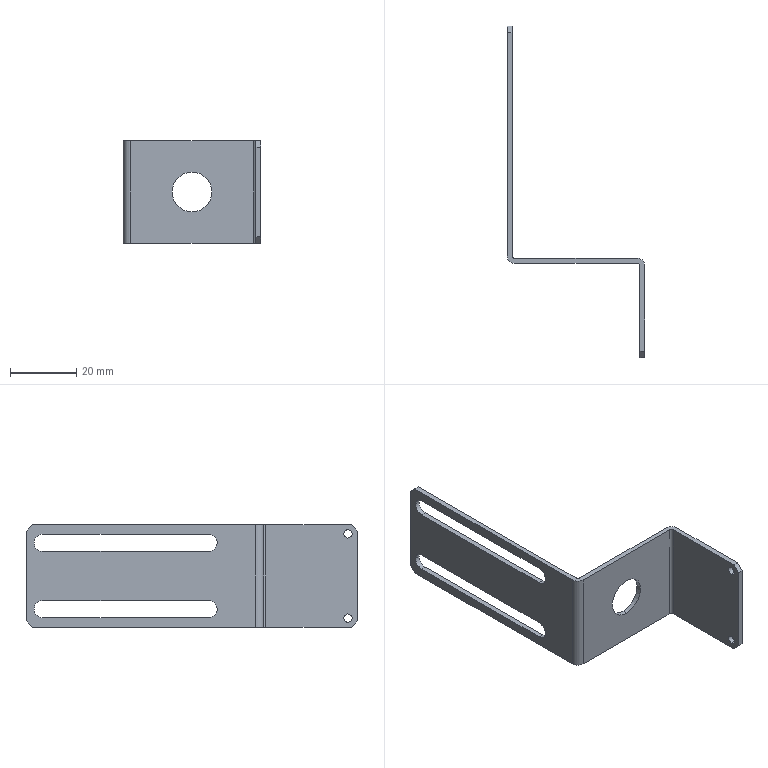Part | SolidWorks | features BaseBody 1 | 1 solid | 34 faces | box 41.5 x 100 x 31 mm | volume 5411 mm3 | plane 18 | cylinder 16 | commonest cylinder face diameters 5.2 x6 2.5 x4 1.473 x2 4.473 x2 12 x2
STEP:
#1=CARTESIAN_POINT('',(40.,-27.,4.05));
#2=VERTEX_POINT('',#1);
#3=CARTESIAN_POINT('',(40.,-27.,1.55));
#4=VERTEX_POINT('',#3);
#5=CARTESIAN_POINT('',(40.,-27.,2.8));
#6=DIRECTION('',(1.,0.,0.));
#7=DIRECTION('',(0.,1.,0.));
#8=AXIS2_PLACEMENT_3D('',#5,#6,#7);
#9=CIRCLE('',#8,1.25);
#10=EDGE_CURVE('',#2,#4,#9,.T.);
#11=ORIENTED_EDGE('',*,*,#10,.T.);
#12=CARTESIAN_POINT('',(38.5,-27.,1.55));
#13=VERTEX_POINT('',#12);
#14=CARTESIAN_POINT('',(38.5,-27.,1.55));
#15=DIRECTION('',(-1.,0.,0.));
#16=VECTOR('',#15,1000.);
#17=LINE('',#14,#16);
#18=EDGE_CURVE('',#4,#13,#17,.T.);
#19=ORIENTED_EDGE('',*,*,#18,.T.);
#20=CARTESIAN_POINT('',(38.5,-27.,4.05));
#21=VERTEX_POINT('',#20);
#22=CARTESIAN_POINT('',(38.5,-27.,2.8));
#23=DIRECTION('',(-1.,0.,0.));
#24=DIRECTION('',(0.,0.,1.));
#25=AXIS2_PLACEMENT_3D('',#22,#23,#24);
#26=CIRCLE('',#25,1.25);
#27=EDGE_CURVE('',#13,#21,#26,.T.);
#28=ORIENTED_EDGE('',*,*,#27,.T.);
#29=CARTESIAN_POINT('',(38.5,-27.,4.05));
#30=DIRECTION('',(-1.,0.,0.));
#31=VECTOR('',#30,1000.);
#32=LINE('',#29,#31);
#33=EDGE_CURVE('',#2,#21,#32,.T.);
#34=ORIENTED_EDGE('',*,*,#33,.F.);
#35=EDGE_LOOP('',(#11,#19,#28,#34));
#36=FACE_OUTER_BOUND('',#35,.T.);
#37=CARTESIAN_POINT('',(38.5,-27.,2.8));
#38=DIRECTION('',(-1.,0.,0.));
#39=DIRECTION('',(0.,0.,1.));
#40=AXIS2_PLACEMENT_3D('',#37,#38,#39);
#41=CYLINDRICAL_SURFACE('',#40,1.25);
#42=ADVANCED_FACE('',(#36),#41,.F.);
#43=CARTESIAN_POINT('',(40.,-27.,29.45));
#44=VERTEX_POINT('',#43);
#45=CARTESIAN_POINT('',(40.,-27.,26.95));
#46=VERTEX_POINT('',#45);
#47=CARTESIAN_POINT('',(40.,-27.,28.2));
#48=DIRECTION('',(1.,0.,0.));
#49=DIRECTION('',(0.,1.,0.));
#50=AXIS2_PLACEMENT_3D('',#47,#48,#49);
#51=CIRCLE('',#50,1.25);
#52=EDGE_CURVE('',#44,#46,#51,.T.);
#53=ORIENTED_EDGE('',*,*,#52,.T.);
#54=CARTESIAN_POINT('',(38.5,-27.,26.95));
#55=VERTEX_POINT('',#54);
#56=CARTESIAN_POINT('',(38.5,-27.,26.95));
#57=DIRECTION('',(-1.,0.,0.));
#58=VECTOR('',#57,1000.);
#59=LINE('',#56,#58);
#60=EDGE_CURVE('',#46,#55,#59,.T.);
#61=ORIENTED_EDGE('',*,*,#60,.T.);
#62=CARTESIAN_POINT('',(38.5,-27.,29.45));
#63=VERTEX_POINT('',#62);
#64=CARTESIAN_POINT('',(38.5,-27.,28.2));
#65=DIRECTION('',(-1.,0.,0.));
#66=DIRECTION('',(0.,0.,1.));
#67=AXIS2_PLACEMENT_3D('',#64,#65,#66);
#68=CIRCLE('',#67,1.25);
#69=EDGE_CURVE('',#55,#63,#68,.T.);
#70=ORIENTED_EDGE('',*,*,#69,.T.);
#71=CARTESIAN_POINT('',(38.5,-27.,29.45));
#72=DIRECTION('',(-1.,0.,0.));
#73=VECTOR('',#72,1000.);
#74=LINE('',#71,#73);
#75=EDGE_CURVE('',#44,#63,#74,.T.);
#76=ORIENTED_EDGE('',*,*,#75,.F.);
#77=EDGE_LOOP('',(#53,#61,#70,#76));
#78=FACE_OUTER_BOUND('',#77,.T.);
#79=CARTESIAN_POINT('',(38.5,-27.,28.2));
#80=DIRECTION('',(-1.,0.,0.));
#81=DIRECTION('',(0.,0.,1.));
#82=AXIS2_PLACEMENT_3D('',#79,#80,#81);
#83=CYLINDRICAL_SURFACE('',#82,1.25);
#84=ADVANCED_FACE('',(#78),#83,.F.);
#85=CARTESIAN_POINT('',(19.25,-1.5,9.5));
#86=VERTEX_POINT('',#85);
#87=CARTESIAN_POINT('',(19.25,-1.5,21.5));
#88=VERTEX_POINT('',#87);
#89=CARTESIAN_POINT('',(19.25,-1.5,15.5));
#90=DIRECTION('',(0.,1.,0.));
#91=DIRECTION('',(0.,0.,1.));
#92=AXIS2_PLACEMENT_3D('',#89,#90,#91);
#93=CIRCLE('',#92,6.);
#94=EDGE_CURVE('',#86,#88,#93,.T.);
#95=ORIENTED_EDGE('',*,*,#94,.F.);
#96=CARTESIAN_POINT('',(19.25,0.,9.5));
#97=VERTEX_POINT('',#96);
#98=CARTESIAN_POINT('',(19.25,-10.,9.5));
#99=DIRECTION('',(0.,1.,0.));
#100=VECTOR('',#99,1000.);
#101=LINE('',#98,#100);
#102=EDGE_CURVE('',#86,#97,#101,.T.);
#103=ORIENTED_EDGE('',*,*,#102,.T.);
#104=CARTESIAN_POINT('',(19.25,0.,21.5));
#105=VERTEX_POINT('',#104);
#106=CARTESIAN_POINT('',(19.25,0.,15.5));
#107=DIRECTION('',(0.,1.,0.));
#108=DIRECTION('',(0.,0.,1.));
#109=AXIS2_PLACEMENT_3D('',#106,#107,#108);
#110=CIRCLE('',#109,6.);
#111=EDGE_CURVE('',#97,#105,#110,.T.);
#112=ORIENTED_EDGE('',*,*,#111,.T.);
#113=CARTESIAN_POINT('',(19.25,-10.,21.5));
#114=DIRECTION('',(0.,1.,0.));
#115=VECTOR('',#114,1000.);
#116=LINE('',#113,#115);
#117=EDGE_CURVE('',#88,#105,#116,.T.);
#118=ORIENTED_EDGE('',*,*,#117,.F.);
#119=EDGE_LOOP('',(#95,#103,#112,#118));
#120=FACE_OUTER_BOUND('',#119,.T.);
#121=CARTESIAN_POINT('',(19.25,-10.,15.5));
#122=DIRECTION('',(0.,1.,0.));
#123=DIRECTION('',(0.,0.,1.));
#124=AXIS2_PLACEMENT_3D('',#121,#122,#123);
#125=CYLINDRICAL_SURFACE('',#124,6.);
#126=ADVANCED_FACE('',(#120),#125,.F.);
#127=CARTESIAN_POINT('',(-1.5,67.6,5.5));
#128=VERTEX_POINT('',#127);
#129=CARTESIAN_POINT('',(-1.5,65.,8.1));
#130=VERTEX_POINT('',#129);
#131=CARTESIAN_POINT('',(-1.5,65.,5.5));
#132=DIRECTION('',(1.,0.,0.));
#133=DIRECTION('',(0.,1.,0.));
#134=AXIS2_PLACEMENT_3D('',#131,#132,#133);
#135=CIRCLE('',#134,2.6);
#136=EDGE_CURVE('',#128,#130,#135,.T.);
#137=ORIENTED_EDGE('',*,*,#136,.F.);
#138=CARTESIAN_POINT('',(0.,67.6,5.5));
#139=VERTEX_POINT('',#138);
#140=CARTESIAN_POINT('',(-10.,67.6,5.5));
#141=DIRECTION('',(1.,0.,0.));
#142=VECTOR('',#141,1000.);
#143=LINE('',#140,#142);
#144=EDGE_CURVE('',#128,#139,#143,.T.);
#145=ORIENTED_EDGE('',*,*,#144,.T.);
#146=CARTESIAN_POINT('',(0.,65.,8.1));
#147=VERTEX_POINT('',#146);
#148=CARTESIAN_POINT('',(0.,65.,5.5));
#149=DIRECTION('',(1.,0.,0.));
#150=DIRECTION('',(0.,1.,0.));
#151=AXIS2_PLACEMENT_3D('',#148,#149,#150);
#152=CIRCLE('',#151,2.6);
#153=EDGE_CURVE('',#139,#147,#152,.T.);
#154=ORIENTED_EDGE('',*,*,#153,.T.);
#155=CARTESIAN_POINT('',(-10.,65.,8.1));
#156=DIRECTION('',(1.,0.,0.));
#157=VECTOR('',#156,1000.);
#158=LINE('',#155,#157);
#159=EDGE_CURVE('',#130,#147,#158,.T.);
#160=ORIENTED_EDGE('',*,*,#159,.F.);
#161=EDGE_LOOP('',(#137,#145,#154,#160));
#162=FACE_OUTER_BOUND('',#161,.T.);
#163=CARTESIAN_POINT('',(-10.,65.,5.5));
#164=DIRECTION('',(1.,0.,0.));
#165=DIRECTION('',(0.,1.,0.));
#166=AXIS2_PLACEMENT_3D('',#163,#164,#165);
#167=CYLINDRICAL_SURFACE('',#166,2.6);
#168=ADVANCED_FACE('',(#162),#167,.F.);
#169=CARTESIAN_POINT('',(-1.5,67.6,25.5));
#170=VERTEX_POINT('',#169);
#171=CARTESIAN_POINT('',(-1.5,65.,28.1));
#172=VERTEX_POINT('',#171);
#173=CARTESIAN_POINT('',(-1.5,65.,25.5));
#174=DIRECTION('',(1.,0.,0.));
#175=DIRECTION('',(0.,1.,0.));
#176=AXIS2_PLACEMENT_3D('',#173,#174,#175);
#177=CIRCLE('',#176,2.6);
#178=EDGE_CURVE('',#170,#172,#177,.T.);
#179=ORIENTED_EDGE('',*,*,#178,.F.);
#180=CARTESIAN_POINT('',(0.,67.6,25.5));
#181=VERTEX_POINT('',#180);
#182=CARTESIAN_POINT('',(-10.,67.6,25.5));
#183=DIRECTION('',(1.,0.,0.));
#184=VECTOR('',#183,1000.);
#185=LINE('',#182,#184);
#186=EDGE_CURVE('',#170,#181,#185,.T.);
#187=ORIENTED_EDGE('',*,*,#186,.T.);
#188=CARTESIAN_POINT('',(0.,65.,28.1));
#189=VERTEX_POINT('',#188);
#190=CARTESIAN_POINT('',(0.,65.,25.5));
#191=DIRECTION('',(1.,0.,0.));
#192=DIRECTION('',(0.,1.,0.));
#193=AXIS2_PLACEMENT_3D('',#190,#191,#192);
#194=CIRCLE('',#193,2.6);
#195=EDGE_CURVE('',#181,#189,#194,.T.);
#196=ORIENTED_EDGE('',*,*,#195,.T.);
#197=CARTESIAN_POINT('',(-10.,65.,28.1));
#198=DIRECTION('',(1.,0.,0.));
#199=VECTOR('',#198,1000.);
#200=LINE('',#197,#199);
#201=EDGE_CURVE('',#172,#189,#200,.T.);
#202=ORIENTED_EDGE('',*,*,#201,.F.);
#203=EDGE_LOOP('',(#179,#187,#196,#202));
#204=FACE_OUTER_BOUND('',#203,.T.);
#205=CARTESIAN_POINT('',(-10.,65.,25.5));
#206=DIRECTION('',(1.,0.,0.));
#207=DIRECTION('',(0.,1.,0.));
#208=AXIS2_PLACEMENT_3D('',#205,#206,#207);
#209=CYLINDRICAL_SURFACE('',#208,2.6);
#210=ADVANCED_FACE('',(#204),#209,.F.);
#211=CARTESIAN_POINT('',(40.,-28.,31.));
#212=VERTEX_POINT('',#211);
#213=CARTESIAN_POINT('',(40.,-30.,29.));
#214=VERTEX_POINT('',#213);
#215=CARTESIAN_POINT('',(40.,-14.,45.));
#216=DIRECTION('',(0.,-0.7071,-0.7071));
#217=VECTOR('',#216,1000.);
#218=LINE('',#215,#217);
#219=EDGE_CURVE('',#212,#214,#218,.T.);
#220=ORIENTED_EDGE('',*,*,#219,.F.);
#221=CARTESIAN_POINT('',(38.5,-28.,31.));
#222=VERTEX_POINT('',#221);
#223=CARTESIAN_POINT('',(37.763,-28.,31.));
#224=DIRECTION('',(1.,0.,0.));
#225=VECTOR('',#224,1000.);
#226=LINE('',#223,#225);
#227=EDGE_CURVE('',#222,#212,#226,.T.);
#228=ORIENTED_EDGE('',*,*,#227,.F.);
#229=CARTESIAN_POINT('',(38.5,-30.,29.));
#230=VERTEX_POINT('',#229);
#231=CARTESIAN_POINT('',(38.5,-30.,29.));
#232=DIRECTION('',(0.,0.7071,0.7071));
#233=VECTOR('',#232,1000.);
#234=LINE('',#231,#233);
#235=EDGE_CURVE('',#230,#222,#234,.T.);
#236=ORIENTED_EDGE('',*,*,#235,.F.);
#237=CARTESIAN_POINT('',(40.,-30.,29.));
#238=DIRECTION('',(-1.,0.,0.));
#239=VECTOR('',#238,1000.);
#240=LINE('',#237,#239);
#241=EDGE_CURVE('',#214,#230,#240,.T.);
#242=ORIENTED_EDGE('',*,*,#241,.F.);
#243=EDGE_LOOP('',(#220,#228,#236,#242));
#244=FACE_OUTER_BOUND('',#243,.T.);
#245=CARTESIAN_POINT('',(40.,-30.,29.));
#246=DIRECTION('',(0.,0.7071,-0.7071));
#247=DIRECTION('',(-1.,0.,0.));
#248=AXIS2_PLACEMENT_3D('',#245,#246,#247);
#249=PLANE('',#248);
#250=ADVANCED_FACE('',(#244),#249,.F.);
#251=CARTESIAN_POINT('',(40.,-30.,2.));
#252=VERTEX_POINT('',#251);
#253=CARTESIAN_POINT('',(40.,-28.,0.));
#254=VERTEX_POINT('',#253);
#255=CARTESIAN_POINT('',(40.,-29.5,1.5));
#256=DIRECTION('',(0.,0.7071,-0.7071));
#257=VECTOR('',#256,1000.);
#258=LINE('',#255,#257);
#259=EDGE_CURVE('',#252,#254,#258,.T.);
#260=ORIENTED_EDGE('',*,*,#259,.F.);
#261=CARTESIAN_POINT('',(38.5,-30.,2.));
#262=VERTEX_POINT('',#261);
#263=CARTESIAN_POINT('',(40.,-30.,2.));
#264=DIRECTION('',(1.,0.,0.));
#265=VECTOR('',#264,1000.);
#266=LINE('',#263,#265);
#267=EDGE_CURVE('',#262,#252,#266,.T.);
#268=ORIENTED_EDGE('',*,*,#267,.F.);
#269=CARTESIAN_POINT('',(38.5,-28.,0.));
#270=VERTEX_POINT('',#269);
#271=CARTESIAN_POINT('',(38.5,-28.,0.));
#272=DIRECTION('',(0.,-0.7071,0.7071));
#273=VECTOR('',#272,1000.);
#274=LINE('',#271,#273);
#275=EDGE_CURVE('',#270,#262,#274,.T.);
#276=ORIENTED_EDGE('',*,*,#275,.F.);
#277=CARTESIAN_POINT('',(38.5,-28.,0.));
#278=DIRECTION('',(-1.,0.,0.));
#279=VECTOR('',#278,1000.);
#280=LINE('',#277,#279);
#281=EDGE_CURVE('',#254,#270,#280,.T.);
#282=ORIENTED_EDGE('',*,*,#281,.F.);
#283=EDGE_LOOP('',(#260,#268,#276,#282));
#284=FACE_OUTER_BOUND('',#283,.T.);
#285=CARTESIAN_POINT('',(37.763,-28.,0.));
#286=DIRECTION('',(0.,-0.7071,-0.7071));
#287=DIRECTION('',(0.,-0.7071,0.7071));
#288=AXIS2_PLACEMENT_3D('',#285,#286,#287);
#289=PLANE('',#288);
#290=ADVANCED_FACE('',(#284),#289,.T.);
#291=CARTESIAN_POINT('',(-1.5,68.,31.));
#292=VERTEX_POINT('',#291);
#293=CARTESIAN_POINT('',(-1.5,70.,29.));
#294=VERTEX_POINT('',#293);
#295=CARTESIAN_POINT('',(-1.5,70.,29.));
#296=DIRECTION('',(0.,0.7071,-0.7071));
#297=VECTOR('',#296,1000.);
#298=LINE('',#295,#297);
#299=EDGE_CURVE('',#292,#294,#298,.T.);
#300=ORIENTED_EDGE('',*,*,#299,.F.);
#301=CARTESIAN_POINT('',(0.,68.,31.));
#302=VERTEX_POINT('',#301);
#303=CARTESIAN_POINT('',(37.763,68.,31.));
#304=DIRECTION('',(-1.,0.,0.));
#305=VECTOR('',#304,1000.);
#306=LINE('',#303,#305);
#307=EDGE_CURVE('',#302,#292,#306,.T.);
#308=ORIENTED_EDGE('',*,*,#307,.F.);
#309=CARTESIAN_POINT('',(0.,70.,29.));
#310=VERTEX_POINT('',#309);
#311=CARTESIAN_POINT('',(0.,69.,30.));
#312=DIRECTION('',(0.,-0.7071,0.7071));
#313=VECTOR('',#312,1000.);
#314=LINE('',#311,#313);
#315=EDGE_CURVE('',#310,#302,#314,.T.);
#316=ORIENTED_EDGE('',*,*,#315,.F.);
#317=CARTESIAN_POINT('',(-1.5,70.,29.));
#318=DIRECTION('',(1.,0.,0.));
#319=VECTOR('',#318,1000.);
#320=LINE('',#317,#319);
#321=EDGE_CURVE('',#294,#310,#320,.T.);
#322=ORIENTED_EDGE('',*,*,#321,.F.);
#323=EDGE_LOOP('',(#300,#308,#316,#322));
#324=FACE_OUTER_BOUND('',#323,.T.);
#325=CARTESIAN_POINT('',(-1.5,70.,29.));
#326=DIRECTION('',(0.,-0.7071,-0.7071));
#327=DIRECTION('',(0.,-0.7071,0.7071));
#328=AXIS2_PLACEMENT_3D('',#325,#326,#327);
#329=PLANE('',#328);
#330=ADVANCED_FACE('',(#324),#329,.F.);
#331=CARTESIAN_POINT('',(-1.5,70.,2.));
#332=VERTEX_POINT('',#331);
#333=CARTESIAN_POINT('',(-1.5,68.,0.));
#334=VERTEX_POINT('',#333);
#335=CARTESIAN_POINT('',(-1.5,68.,0.));
#336=DIRECTION('',(0.,-0.7071,-0.7071));
#337=VECTOR('',#336,1000.);
#338=LINE('',#335,#337);
#339=EDGE_CURVE('',#332,#334,#338,.T.);
#340=ORIENTED_EDGE('',*,*,#339,.F.);
#341=CARTESIAN_POINT('',(0.,70.,2.));
#342=VERTEX_POINT('',#341);
#343=CARTESIAN_POINT('',(-1.5,70.,2.));
#344=DIRECTION('',(-1.,0.,0.));
#345=VECTOR('',#344,1000.);
#346=LINE('',#343,#345);
#347=EDGE_CURVE('',#342,#332,#346,.T.);
#348=ORIENTED_EDGE('',*,*,#347,.F.);
#349=CARTESIAN_POINT('',(0.,68.,0.));
#350=VERTEX_POINT('',#349);
#351=CARTESIAN_POINT('',(0.,84.5,16.5));
#352=DIRECTION('',(0.,0.7071,0.7071));
#353=VECTOR('',#352,1000.);
#354=LINE('',#351,#353);
#355=EDGE_CURVE('',#350,#342,#354,.T.);
#356=ORIENTED_EDGE('',*,*,#355,.F.);
#357=CARTESIAN_POINT('',(0.7366,68.,0.));
#358=DIRECTION('',(1.,0.,0.));
#359=VECTOR('',#358,1000.);
#360=LINE('',#357,#359);
#361=EDGE_CURVE('',#334,#350,#360,.T.);
#362=ORIENTED_EDGE('',*,*,#361,.F.);
#363=EDGE_LOOP('',(#340,#348,#356,#362));
#364=FACE_OUTER_BOUND('',#363,.T.);
#365=CARTESIAN_POINT('',(0.7366,68.,0.));
#366=DIRECTION('',(0.,-0.7071,0.7071));
#367=DIRECTION('',(-1.,0.,0.));
#368=AXIS2_PLACEMENT_3D('',#365,#366,#367);
#369=PLANE('',#368);
#370=ADVANCED_FACE('',(#364),#369,.F.);
#371=ORIENTED_EDGE('',*,*,#159,.T.);
#372=CARTESIAN_POINT('',(0.,15.,8.1));
#373=VERTEX_POINT('',#372);
#374=CARTESIAN_POINT('',(0.,65.,8.1));
#375=DIRECTION('',(0.,-1.,0.));
#376=VECTOR('',#375,1000.);
#377=LINE('',#374,#376);
#378=EDGE_CURVE('',#147,#373,#377,.T.);
#379=ORIENTED_EDGE('',*,*,#378,.T.);
#380=CARTESIAN_POINT('',(-1.5,15.,8.1));
#381=VERTEX_POINT('',#380);
#382=CARTESIAN_POINT('',(-10.,15.,8.1));
#383=DIRECTION('',(1.,0.,0.));
#384=VECTOR('',#383,1000.);
#385=LINE('',#382,#384);
#386=EDGE_CURVE('',#381,#373,#385,.T.);
#387=ORIENTED_EDGE('',*,*,#386,.F.);
#388=CARTESIAN_POINT('',(-1.5,70.,8.1));
#389=DIRECTION('',(0.,-1.,0.));
#390=VECTOR('',#389,1000.);
#391=LINE('',#388,#390);
#392=EDGE_CURVE('',#130,#381,#391,.T.);
#393=ORIENTED_EDGE('',*,*,#392,.F.);
#394=EDGE_LOOP('',(#371,#379,#387,#393));
#395=FACE_OUTER_BOUND('',#394,.T.);
#396=CARTESIAN_POINT('',(-10.,65.,8.1));
#397=DIRECTION('',(0.,0.,1.));
#398=DIRECTION('',(0.,-1.,0.));
#399=AXIS2_PLACEMENT_3D('',#396,#397,#398);
#400=PLANE('',#399);
#401=ADVANCED_FACE('',(#395),#400,.F.);
#402=ORIENTED_EDGE('',*,*,#386,.T.);
#403=CARTESIAN_POINT('',(0.,15.,2.9));
#404=VERTEX_POINT('',#403);
#405=CARTESIAN_POINT('',(0.,15.,5.5));
#406=DIRECTION('',(1.,0.,0.));
#407=DIRECTION('',(0.,1.,0.));
#408=AXIS2_PLACEMENT_3D('',#405,#406,#407);
#409=CIRCLE('',#408,2.6);
#410=EDGE_CURVE('',#373,#404,#409,.T.);
#411=ORIENTED_EDGE('',*,*,#410,.T.);
#412=CARTESIAN_POINT('',(-1.5,15.,2.9));
#413=VERTEX_POINT('',#412);
#414=CARTESIAN_POINT('',(-10.,15.,2.9));
#415=DIRECTION('',(1.,0.,0.));
#416=VECTOR('',#415,1000.);
#417=LINE('',#414,#416);
#418=EDGE_CURVE('',#413,#404,#417,.T.);
#419=ORIENTED_EDGE('',*,*,#418,.F.);
#420=CARTESIAN_POINT('',(-1.5,15.,5.5));
#421=DIRECTION('',(1.,0.,0.));
#422=DIRECTION('',(0.,1.,0.));
#423=AXIS2_PLACEMENT_3D('',#420,#421,#422);
#424=CIRCLE('',#423,2.6);
#425=EDGE_CURVE('',#381,#413,#424,.T.);
#426=ORIENTED_EDGE('',*,*,#425,.F.);
#427=EDGE_LOOP('',(#402,#411,#419,#426));
#428=FACE_OUTER_BOUND('',#427,.T.);
#429=CARTESIAN_POINT('',(-10.,15.,5.5));
#430=DIRECTION('',(1.,0.,0.));
#431=DIRECTION('',(0.,1.,0.));
#432=AXIS2_PLACEMENT_3D('',#429,#430,#431);
#433=CYLINDRICAL_SURFACE('',#432,2.6);
#434=ADVANCED_FACE('',(#428),#433,.F.);
#435=ORIENTED_EDGE('',*,*,#418,.T.);
#436=CARTESIAN_POINT('',(0.,65.,2.9));
#437=VERTEX_POINT('',#436);
#438=CARTESIAN_POINT('',(0.,65.,2.9));
#439=DIRECTION('',(0.,1.,0.));
#440=VECTOR('',#439,1000.);
#441=LINE('',#438,#440);
#442=EDGE_CURVE('',#404,#437,#441,.T.);
#443=ORIENTED_EDGE('',*,*,#442,.T.);
#444=CARTESIAN_POINT('',(-1.5,65.,2.9));
#445=VERTEX_POINT('',#444);
#446=CARTESIAN_POINT('',(-10.,65.,2.9));
#447=DIRECTION('',(1.,0.,0.));
#448=VECTOR('',#447,1000.);
#449=LINE('',#446,#448);
#450=EDGE_CURVE('',#445,#437,#449,.T.);
#451=ORIENTED_EDGE('',*,*,#450,.F.);
#452=CARTESIAN_POINT('',(-1.5,70.,2.9));
#453=DIRECTION('',(0.,1.,0.));
#454=VECTOR('',#453,1000.);
#455=LINE('',#452,#454);
#456=EDGE_CURVE('',#413,#445,#455,.T.);
#457=ORIENTED_EDGE('',*,*,#456,.F.);
#458=EDGE_LOOP('',(#435,#443,#451,#457));
#459=FACE_OUTER_BOUND('',#458,.T.);
#460=CARTESIAN_POINT('',(-10.,65.,2.9));
#461=DIRECTION('',(0.,0.,-1.));
#462=DIRECTION('',(-1.,0.,0.));
#463=AXIS2_PLACEMENT_3D('',#460,#461,#462);
#464=PLANE('',#463);
#465=ADVANCED_FACE('',(#459),#464,.F.);
#466=ORIENTED_EDGE('',*,*,#201,.T.);
#467=CARTESIAN_POINT('',(0.,15.,28.1));
#468=VERTEX_POINT('',#467);
#469=CARTESIAN_POINT('',(0.,65.,28.1));
#470=DIRECTION('',(0.,-1.,0.));
#471=VECTOR('',#470,1000.);
#472=LINE('',#469,#471);
#473=EDGE_CURVE('',#189,#468,#472,.T.);
#474=ORIENTED_EDGE('',*,*,#473,.T.);
#475=CARTESIAN_POINT('',(-1.5,15.,28.1));
#476=VERTEX_POINT('',#475);
#477=CARTESIAN_POINT('',(-10.,15.,28.1));
#478=DIRECTION('',(1.,0.,0.));
#479=VECTOR('',#478,1000.);
#480=LINE('',#477,#479);
#481=EDGE_CURVE('',#476,#468,#480,.T.);
#482=ORIENTED_EDGE('',*,*,#481,.F.);
#483=CARTESIAN_POINT('',(-1.5,70.,28.1));
#484=DIRECTION('',(0.,-1.,0.));
#485=VECTOR('',#484,1000.);
#486=LINE('',#483,#485);
#487=EDGE_CURVE('',#172,#476,#486,.T.);
#488=ORIENTED_EDGE('',*,*,#487,.F.);
#489=EDGE_LOOP('',(#466,#474,#482,#488));
#490=FACE_OUTER_BOUND('',#489,.T.);
#491=CARTESIAN_POINT('',(-10.,65.,28.1));
#492=DIRECTION('',(0.,0.,1.));
#493=DIRECTION('',(0.,-1.,0.));
#494=AXIS2_PLACEMENT_3D('',#491,#492,#493);
#495=PLANE('',#494);
#496=ADVANCED_FACE('',(#490),#495,.F.);
#497=ORIENTED_EDGE('',*,*,#481,.T.);
#498=CARTESIAN_POINT('',(0.,15.,22.9));
#499=VERTEX_POINT('',#498);
#500=CARTESIAN_POINT('',(0.,15.,25.5));
#501=DIRECTION('',(1.,0.,0.));
#502=DIRECTION('',(0.,1.,0.));
#503=AXIS2_PLACEMENT_3D('',#500,#501,#502);
#504=CIRCLE('',#503,2.6);
#505=EDGE_CURVE('',#468,#499,#504,.T.);
#506=ORIENTED_EDGE('',*,*,#505,.T.);
#507=CARTESIAN_POINT('',(-1.5,15.,22.9));
#508=VERTEX_POINT('',#507);
#509=CARTESIAN_POINT('',(-10.,15.,22.9));
#510=DIRECTION('',(1.,0.,0.));
#511=VECTOR('',#510,1000.);
#512=LINE('',#509,#511);
#513=EDGE_CURVE('',#508,#499,#512,.T.);
#514=ORIENTED_EDGE('',*,*,#513,.F.);
#515=CARTESIAN_POINT('',(-1.5,15.,25.5));
#516=DIRECTION('',(1.,0.,0.));
#517=DIRECTION('',(0.,1.,0.));
#518=AXIS2_PLACEMENT_3D('',#515,#516,#517);
#519=CIRCLE('',#518,2.6);
#520=EDGE_CURVE('',#476,#508,#519,.T.);
#521=ORIENTED_EDGE('',*,*,#520,.F.);
#522=EDGE_LOOP('',(#497,#506,#514,#521));
#523=FACE_OUTER_BOUND('',#522,.T.);
#524=CARTESIAN_POINT('',(-10.,15.,25.5));
#525=DIRECTION('',(1.,0.,0.));
#526=DIRECTION('',(0.,1.,0.));
#527=AXIS2_PLACEMENT_3D('',#524,#525,#526);
#528=CYLINDRICAL_SURFACE('',#527,2.6);
#529=ADVANCED_FACE('',(#523),#528,.F.);
#530=ORIENTED_EDGE('',*,*,#513,.T.);
#531=CARTESIAN_POINT('',(0.,65.,22.9));
#532=VERTEX_POINT('',#531);
#533=CARTESIAN_POINT('',(0.,65.,22.9));
#534=DIRECTION('',(0.,1.,0.));
#535=VECTOR('',#534,1000.);
#536=LINE('',#533,#535);
#537=EDGE_CURVE('',#499,#532,#536,.T.);
#538=ORIENTED_EDGE('',*,*,#537,.T.);
#539=CARTESIAN_POINT('',(-1.5,65.,22.9));
#540=VERTEX_POINT('',#539);
#541=CARTESIAN_POINT('',(-10.,65.,22.9));
#542=DIRECTION('',(1.,0.,0.));
#543=VECTOR('',#542,1000.);
#544=LINE('',#541,#543);
#545=EDGE_CURVE('',#540,#532,#544,.T.);
#546=ORIENTED_EDGE('',*,*,#545,.F.);
#547=CARTESIAN_POINT('',(-1.5,70.,22.9));
#548=DIRECTION('',(0.,1.,0.));
#549=VECTOR('',#548,1000.);
#550=LINE('',#547,#549);
#551=EDGE_CURVE('',#508,#540,#550,.T.);
#552=ORIENTED_EDGE('',*,*,#551,.F.);
#553=EDGE_LOOP('',(#530,#538,#546,#552));
#554=FACE_OUTER_BOUND('',#553,.T.);
#555=CARTESIAN_POINT('',(-10.,65.,22.9));
#556=DIRECTION('',(0.,0.,-1.));
#557=DIRECTION('',(-1.,0.,0.));
#558=AXIS2_PLACEMENT_3D('',#555,#556,#557);
#559=PLANE('',#558);
#560=ADVANCED_FACE('',(#554),#559,.F.);
#561=CARTESIAN_POINT('',(37.763,-1.5,0.));
#562=VERTEX_POINT('',#561);
#563=CARTESIAN_POINT('',(38.5,-2.237,0.));
#564=VERTEX_POINT('',#563);
#565=CARTESIAN_POINT('',(37.763,-2.237,0.));
#566=DIRECTION('',(0.,0.,-1.));
#567=DIRECTION('',(1.,0.,0.));
#568=AXIS2_PLACEMENT_3D('',#565,#566,#567);
#569=CIRCLE('',#568,0.7366);
#570=EDGE_CURVE('',#562,#564,#569,.T.);
#571=ORIENTED_EDGE('',*,*,#570,.T.);
#572=CARTESIAN_POINT('',(38.5,-2.237,31.));
#573=VERTEX_POINT('',#572);
#574=CARTESIAN_POINT('',(38.5,-2.237,31.));
#575=DIRECTION('',(0.,0.,-1.));
#576=VECTOR('',#575,1000.);
#577=LINE('',#574,#576);
#578=EDGE_CURVE('',#573,#564,#577,.T.);
#579=ORIENTED_EDGE('',*,*,#578,.F.);
#580=CARTESIAN_POINT('',(37.763,-1.5,31.));
#581=VERTEX_POINT('',#580);
#582=CARTESIAN_POINT('',(37.763,-2.237,31.));
#583=DIRECTION('',(0.,0.,-1.));
#584=DIRECTION('',(1.,0.,0.));
#585=AXIS2_PLACEMENT_3D('',#582,#583,#584);
#586=CIRCLE('',#585,0.7366);
#587=EDGE_CURVE('',#581,#573,#586,.T.);
#588=ORIENTED_EDGE('',*,*,#587,.F.);
#589=CARTESIAN_POINT('',(37.763,-1.5,31.));
#590=DIRECTION('',(0.,0.,-1.));
#591=VECTOR('',#590,1000.);
#592=LINE('',#589,#591);
#593=EDGE_CURVE('',#581,#562,#592,.T.);
#594=ORIENTED_EDGE('',*,*,#593,.T.);
#595=EDGE_LOOP('',(#571,#579,#588,#594));
#596=FACE_OUTER_BOUND('',#595,.T.);
#597=CARTESIAN_POINT('',(37.763,-2.237,31.));
#598=DIRECTION('',(0.,0.,-1.));
#599=DIRECTION('',(-1.,0.,0.));
#600=AXIS2_PLACEMENT_3D('',#597,#598,#599);
#601=CYLINDRICAL_SURFACE('',#600,0.7366);
#602=ADVANCED_FACE('',(#596),#601,.F.);
#603=CARTESIAN_POINT('',(19.25,-1.5,15.5));
#604=DIRECTION('',(0.,1.,0.));
#605=DIRECTION('',(0.,0.,1.));
#606=AXIS2_PLACEMENT_3D('',#603,#604,#605);
#607=CIRCLE('',#606,6.);
#608=EDGE_CURVE('',#88,#86,#607,.T.);
#609=ORIENTED_EDGE('',*,*,#608,.T.);
#610=ORIENTED_EDGE('',*,*,#94,.T.);
#611=EDGE_LOOP('',(#609,#610));
#612=FACE_BOUND('',#611,.T.);
#613=CARTESIAN_POINT('',(0.7366,-1.5,0.));
#614=VERTEX_POINT('',#613);
#615=CARTESIAN_POINT('',(0.,-1.5,0.));
#616=DIRECTION('',(1.,0.,0.));
#617=VECTOR('',#616,1000.);
#618=LINE('',#615,#617);
#619=EDGE_CURVE('',#614,#562,#618,.T.);
#620=ORIENTED_EDGE('',*,*,#619,.T.);
#621=ORIENTED_EDGE('',*,*,#593,.F.);
#622=CARTESIAN_POINT('',(0.7366,-1.5,31.));
#623=VERTEX_POINT('',#622);
#624=CARTESIAN_POINT('',(0.,-1.5,31.));
#625=DIRECTION('',(1.,0.,0.));
#626=VECTOR('',#625,1000.);
#627=LINE('',#624,#626);
#628=EDGE_CURVE('',#623,#581,#627,.T.);
#629=ORIENTED_EDGE('',*,*,#628,.F.);
#630=CARTESIAN_POINT('',(0.7366,-1.5,31.));
#631=DIRECTION('',(0.,0.,-1.));
#632=VECTOR('',#631,1000.);
#633=LINE('',#630,#632);
#634=EDGE_CURVE('',#623,#614,#633,.T.);
#635=ORIENTED_EDGE('',*,*,#634,.T.);
#636=EDGE_LOOP('',(#620,#621,#629,#635));
#637=FACE_OUTER_BOUND('',#636,.T.);
#638=CARTESIAN_POINT('',(0.,-1.5,31.));
#639=DIRECTION('',(0.,1.,0.));
#640=DIRECTION('',(1.,0.,0.));
#641=AXIS2_PLACEMENT_3D('',#638,#639,#640);
#642=PLANE('',#641);
#643=ADVANCED_FACE('',(#612,#637),#642,.F.);
#644=CARTESIAN_POINT('',(-1.5,0.7366,0.));
#645=VERTEX_POINT('',#644);
#646=CARTESIAN_POINT('',(0.7366,0.7366,0.));
#647=DIRECTION('',(0.,0.,1.));
#648=DIRECTION('',(1.,0.,0.));
#649=AXIS2_PLACEMENT_3D('',#646,#647,#648);
#650=CIRCLE('',#649,2.237);
#651=EDGE_CURVE('',#645,#614,#650,.T.);
#652=ORIENTED_EDGE('',*,*,#651,.T.);
#653=ORIENTED_EDGE('',*,*,#634,.F.);
#654=CARTESIAN_POINT('',(-1.5,0.7366,31.));
#655=VERTEX_POINT('',#654);
#656=CARTESIAN_POINT('',(0.7366,0.7366,31.));
#657=DIRECTION('',(0.,0.,1.));
#658=DIRECTION('',(1.,0.,0.));
#659=AXIS2_PLACEMENT_3D('',#656,#657,#658);
#660=CIRCLE('',#659,2.237);
#661=EDGE_CURVE('',#655,#623,#660,.T.);
#662=ORIENTED_EDGE('',*,*,#661,.F.);
#663=CARTESIAN_POINT('',(-1.5,0.7366,31.));
#664=DIRECTION('',(0.,0.,-1.));
#665=VECTOR('',#664,1000.);
#666=LINE('',#663,#665);
#667=EDGE_CURVE('',#655,#645,#666,.T.);
#668=ORIENTED_EDGE('',*,*,#667,.T.);
#669=EDGE_LOOP('',(#652,#653,#662,#668));
#670=FACE_OUTER_BOUND('',#669,.T.);
#671=CARTESIAN_POINT('',(0.7366,0.7366,31.));
#672=DIRECTION('',(0.,0.,-1.));
#673=DIRECTION('',(-1.,0.,0.));
#674=AXIS2_PLACEMENT_3D('',#671,#672,#673);
#675=CYLINDRICAL_SURFACE('',#674,2.237);
#676=ADVANCED_FACE('',(#670),#675,.T.);
#677=ORIENTED_EDGE('',*,*,#551,.T.);
#678=CARTESIAN_POINT('',(-1.5,65.,25.5));
#679=DIRECTION('',(1.,0.,0.));
#680=DIRECTION('',(0.,1.,0.));
#681=AXIS2_PLACEMENT_3D('',#678,#679,#680);
#682=CIRCLE('',#681,2.6);
#683=EDGE_CURVE('',#540,#170,#682,.T.);
#684=ORIENTED_EDGE('',*,*,#683,.T.);
#685=ORIENTED_EDGE('',*,*,#178,.T.);
#686=ORIENTED_EDGE('',*,*,#487,.T.);
#687=ORIENTED_EDGE('',*,*,#520,.T.);
#688=EDGE_LOOP('',(#677,#684,#685,#686,#687));
#689=FACE_BOUND('',#688,.T.);
#690=ORIENTED_EDGE('',*,*,#456,.T.);
#691=CARTESIAN_POINT('',(-1.5,65.,5.5));
#692=DIRECTION('',(1.,0.,0.));
#693=DIRECTION('',(0.,1.,0.));
#694=AXIS2_PLACEMENT_3D('',#691,#692,#693);
#695=CIRCLE('',#694,2.6);
#696=EDGE_CURVE('',#445,#128,#695,.T.);
#697=ORIENTED_EDGE('',*,*,#696,.T.);
#698=ORIENTED_EDGE('',*,*,#136,.T.);
#699=ORIENTED_EDGE('',*,*,#392,.T.);
#700=ORIENTED_EDGE('',*,*,#425,.T.);
#701=EDGE_LOOP('',(#690,#697,#698,#699,#700));
#702=FACE_BOUND('',#701,.T.);
#703=CARTESIAN_POINT('',(-1.5,70.,31.));
#704=DIRECTION('',(0.,0.,-1.));
#705=VECTOR('',#704,1000.);
#706=LINE('',#703,#705);
#707=EDGE_CURVE('',#294,#332,#706,.T.);
#708=ORIENTED_EDGE('',*,*,#707,.T.);
#709=ORIENTED_EDGE('',*,*,#339,.T.);
#710=CARTESIAN_POINT('',(-1.5,70.,0.));
#711=DIRECTION('',(0.,-1.,0.));
#712=VECTOR('',#711,1000.);
#713=LINE('',#710,#712);
#714=EDGE_CURVE('',#334,#645,#713,.T.);
#715=ORIENTED_EDGE('',*,*,#714,.T.);
#716=ORIENTED_EDGE('',*,*,#667,.F.);
#717=CARTESIAN_POINT('',(-1.5,70.,31.));
#718=DIRECTION('',(0.,-1.,0.));
#719=VECTOR('',#718,1000.);
#720=LINE('',#717,#719);
#721=EDGE_CURVE('',#292,#655,#720,.T.);
#722=ORIENTED_EDGE('',*,*,#721,.F.);
#723=ORIENTED_EDGE('',*,*,#299,.T.);
#724=EDGE_LOOP('',(#708,#709,#715,#716,#722,#723));
#725=FACE_OUTER_BOUND('',#724,.T.);
#726=CARTESIAN_POINT('',(-1.5,70.,31.));
#727=DIRECTION('',(1.,0.,0.));
#728=DIRECTION('',(0.,-1.,0.));
#729=AXIS2_PLACEMENT_3D('',#726,#727,#728);
#730=PLANE('',#729);
#731=ADVANCED_FACE('',(#689,#702,#725),#730,.F.);
#732=CARTESIAN_POINT('',(0.,70.,31.));
#733=DIRECTION('',(0.,0.,-1.));
#734=VECTOR('',#733,1000.);
#735=LINE('',#732,#734);
#736=EDGE_CURVE('',#310,#342,#735,.T.);
#737=ORIENTED_EDGE('',*,*,#736,.T.);
#738=ORIENTED_EDGE('',*,*,#347,.T.);
#739=ORIENTED_EDGE('',*,*,#707,.F.);
#740=ORIENTED_EDGE('',*,*,#321,.T.);
#741=EDGE_LOOP('',(#737,#738,#739,#740));
#742=FACE_OUTER_BOUND('',#741,.T.);
#743=CARTESIAN_POINT('',(-1.5,70.,31.));
#744=DIRECTION('',(0.,1.,0.));
#745=DIRECTION('',(1.,0.,0.));
#746=AXIS2_PLACEMENT_3D('',#743,#744,#745);
#747=PLANE('',#746);
#748=ADVANCED_FACE('',(#742),#747,.T.);
#749=CARTESIAN_POINT('',(0.,65.,25.5));
#750=DIRECTION('',(1.,0.,0.));
#751=DIRECTION('',(0.,1.,0.));
#752=AXIS2_PLACEMENT_3D('',#749,#750,#751);
#753=CIRCLE('',#752,2.6);
#754=EDGE_CURVE('',#532,#181,#753,.T.);
#755=ORIENTED_EDGE('',*,*,#754,.F.);
#756=ORIENTED_EDGE('',*,*,#537,.F.);
#757=ORIENTED_EDGE('',*,*,#505,.F.);
#758=ORIENTED_EDGE('',*,*,#473,.F.);
#759=ORIENTED_EDGE('',*,*,#195,.F.);
#760=EDGE_LOOP('',(#755,#756,#757,#758,#759));
#761=FACE_BOUND('',#760,.T.);
#762=CARTESIAN_POINT('',(0.,65.,5.5));
#763=DIRECTION('',(1.,0.,0.));
#764=DIRECTION('',(0.,1.,0.));
#765=AXIS2_PLACEMENT_3D('',#762,#763,#764);
#766=CIRCLE('',#765,2.6);
#767=EDGE_CURVE('',#437,#139,#766,.T.);
#768=ORIENTED_EDGE('',*,*,#767,.F.);
#769=ORIENTED_EDGE('',*,*,#442,.F.);
#770=ORIENTED_EDGE('',*,*,#410,.F.);
#771=ORIENTED_EDGE('',*,*,#378,.F.);
#772=ORIENTED_EDGE('',*,*,#153,.F.);
#773=EDGE_LOOP('',(#768,#769,#770,#771,#772));
#774=FACE_BOUND('',#773,.T.);
#775=CARTESIAN_POINT('',(0.,0.7366,0.));
#776=VERTEX_POINT('',#775);
#777=CARTESIAN_POINT('',(0.,70.,0.));
#778=DIRECTION('',(0.,-1.,0.));
#779=VECTOR('',#778,1000.);
#780=LINE('',#777,#779);
#781=EDGE_CURVE('',#350,#776,#780,.T.);
#782=ORIENTED_EDGE('',*,*,#781,.F.);
#783=ORIENTED_EDGE('',*,*,#355,.T.);
#784=ORIENTED_EDGE('',*,*,#736,.F.);
#785=ORIENTED_EDGE('',*,*,#315,.T.);
#786=CARTESIAN_POINT('',(0.,0.7366,31.));
#787=VERTEX_POINT('',#786);
#788=CARTESIAN_POINT('',(0.,70.,31.));
#789=DIRECTION('',(0.,-1.,0.));
#790=VECTOR('',#789,1000.);
#791=LINE('',#788,#790);
#792=EDGE_CURVE('',#302,#787,#791,.T.);
#793=ORIENTED_EDGE('',*,*,#792,.T.);
#794=CARTESIAN_POINT('',(0.,0.7366,31.));
#795=DIRECTION('',(0.,0.,-1.));
#796=VECTOR('',#795,1000.);
#797=LINE('',#794,#796);
#798=EDGE_CURVE('',#787,#776,#797,.T.);
#799=ORIENTED_EDGE('',*,*,#798,.T.);
#800=EDGE_LOOP('',(#782,#783,#784,#785,#793,#799));
#801=FACE_OUTER_BOUND('',#800,.T.);
#802=CARTESIAN_POINT('',(0.,70.,31.));
#803=DIRECTION('',(1.,0.,0.));
#804=DIRECTION('',(0.,-1.,0.));
#805=AXIS2_PLACEMENT_3D('',#802,#803,#804);
#806=PLANE('',#805);
#807=ADVANCED_FACE('',(#761,#774,#801),#806,.T.);
#808=CARTESIAN_POINT('',(0.7366,0.,0.));
#809=VERTEX_POINT('',#808);
#810=CARTESIAN_POINT('',(0.7366,0.7366,0.));
#811=DIRECTION('',(0.,0.,1.));
#812=DIRECTION('',(-1.,0.,0.));
#813=AXIS2_PLACEMENT_3D('',#810,#811,#812);
#814=CIRCLE('',#813,0.7366);
#815=EDGE_CURVE('',#776,#809,#814,.T.);
#816=ORIENTED_EDGE('',*,*,#815,.F.);
#817=ORIENTED_EDGE('',*,*,#798,.F.);
#818=CARTESIAN_POINT('',(0.7366,0.,31.));
#819=VERTEX_POINT('',#818);
#820=CARTESIAN_POINT('',(0.7366,0.7366,31.));
#821=DIRECTION('',(0.,0.,1.));
#822=DIRECTION('',(-1.,0.,0.));
#823=AXIS2_PLACEMENT_3D('',#820,#821,#822);
#824=CIRCLE('',#823,0.7366);
#825=EDGE_CURVE('',#787,#819,#824,.T.);
#826=ORIENTED_EDGE('',*,*,#825,.T.);
#827=CARTESIAN_POINT('',(0.7366,0.,31.));
#828=DIRECTION('',(0.,0.,-1.));
#829=VECTOR('',#828,1000.);
#830=LINE('',#827,#829);
#831=EDGE_CURVE('',#819,#809,#830,.T.);
#832=ORIENTED_EDGE('',*,*,#831,.T.);
#833=EDGE_LOOP('',(#816,#817,#826,#832));
#834=FACE_OUTER_BOUND('',#833,.T.);
#835=CARTESIAN_POINT('',(0.7366,0.7366,31.));
#836=DIRECTION('',(0.,0.,-1.));
#837=DIRECTION('',(-1.,0.,0.));
#838=AXIS2_PLACEMENT_3D('',#835,#836,#837);
#839=CYLINDRICAL_SURFACE('',#838,0.7366);
#840=ADVANCED_FACE('',(#834),#839,.F.);
#841=CARTESIAN_POINT('',(19.25,0.,15.5));
#842=DIRECTION('',(0.,1.,0.));
#843=DIRECTION('',(0.,0.,1.));
#844=AXIS2_PLACEMENT_3D('',#841,#842,#843);
#845=CIRCLE('',#844,6.);
#846=EDGE_CURVE('',#105,#97,#845,.T.);
#847=ORIENTED_EDGE('',*,*,#846,.F.);
#848=ORIENTED_EDGE('',*,*,#111,.F.);
#849=EDGE_LOOP('',(#847,#848));
#850=FACE_BOUND('',#849,.T.);
#851=CARTESIAN_POINT('',(37.763,0.,0.));
#852=VERTEX_POINT('',#851);
#853=CARTESIAN_POINT('',(0.,0.,0.));
#854=DIRECTION('',(1.,0.,0.));
#855=VECTOR('',#854,1000.);
#856=LINE('',#853,#855);
#857=EDGE_CURVE('',#809,#852,#856,.T.);
#858=ORIENTED_EDGE('',*,*,#857,.F.);
#859=ORIENTED_EDGE('',*,*,#831,.F.);
#860=CARTESIAN_POINT('',(37.763,0.,31.));
#861=VERTEX_POINT('',#860);
#862=CARTESIAN_POINT('',(0.,0.,31.));
#863=DIRECTION('',(1.,0.,0.));
#864=VECTOR('',#863,1000.);
#865=LINE('',#862,#864);
#866=EDGE_CURVE('',#819,#861,#865,.T.);
#867=ORIENTED_EDGE('',*,*,#866,.T.);
#868=CARTESIAN_POINT('',(37.763,0.,31.));
#869=DIRECTION('',(0.,0.,-1.));
#870=VECTOR('',#869,1000.);
#871=LINE('',#868,#870);
#872=EDGE_CURVE('',#861,#852,#871,.T.);
#873=ORIENTED_EDGE('',*,*,#872,.T.);
#874=EDGE_LOOP('',(#858,#859,#867,#873));
#875=FACE_OUTER_BOUND('',#874,.T.);
#876=CARTESIAN_POINT('',(0.,0.,31.));
#877=DIRECTION('',(0.,1.,0.));
#878=DIRECTION('',(1.,0.,0.));
#879=AXIS2_PLACEMENT_3D('',#876,#877,#878);
#880=PLANE('',#879);
#881=ADVANCED_FACE('',(#850,#875),#880,.T.);
#882=CARTESIAN_POINT('',(40.,-2.237,0.));
#883=VERTEX_POINT('',#882);
#884=CARTESIAN_POINT('',(37.763,-2.237,0.));
#885=DIRECTION('',(0.,0.,-1.));
#886=DIRECTION('',(1.,0.,0.));
#887=AXIS2_PLACEMENT_3D('',#884,#885,#886);
#888=CIRCLE('',#887,2.237);
#889=EDGE_CURVE('',#852,#883,#888,.T.);
#890=ORIENTED_EDGE('',*,*,#889,.F.);
#891=ORIENTED_EDGE('',*,*,#872,.F.);
#892=CARTESIAN_POINT('',(40.,-2.237,31.));
#893=VERTEX_POINT('',#892);
#894=CARTESIAN_POINT('',(37.763,-2.237,31.));
#895=DIRECTION('',(0.,0.,-1.));
#896=DIRECTION('',(1.,0.,0.));
#897=AXIS2_PLACEMENT_3D('',#894,#895,#896);
#898=CIRCLE('',#897,2.237);
#899=EDGE_CURVE('',#861,#893,#898,.T.);
#900=ORIENTED_EDGE('',*,*,#899,.T.);
#901=CARTESIAN_POINT('',(40.,-2.237,31.));
#902=DIRECTION('',(0.,0.,-1.));
#903=VECTOR('',#902,1000.);
#904=LINE('',#901,#903);
#905=EDGE_CURVE('',#893,#883,#904,.T.);
#906=ORIENTED_EDGE('',*,*,#905,.T.);
#907=EDGE_LOOP('',(#890,#891,#900,#906));
#908=FACE_OUTER_BOUND('',#907,.T.);
#909=CARTESIAN_POINT('',(37.763,-2.237,31.));
#910=DIRECTION('',(0.,0.,-1.));
#911=DIRECTION('',(-1.,0.,0.));
#912=AXIS2_PLACEMENT_3D('',#909,#910,#911);
#913=CYLINDRICAL_SURFACE('',#912,2.237);
#914=ADVANCED_FACE('',(#908),#913,.T.);
#915=ORIENTED_EDGE('',*,*,#52,.F.);
#916=CARTESIAN_POINT('',(40.,-27.,28.2));
#917=DIRECTION('',(1.,0.,0.));
#918=DIRECTION('',(0.,1.,0.));
#919=AXIS2_PLACEMENT_3D('',#916,#917,#918);
#920=CIRCLE('',#919,1.25);
#921=EDGE_CURVE('',#46,#44,#920,.T.);
#922=ORIENTED_EDGE('',*,*,#921,.F.);
#923=EDGE_LOOP('',(#915,#922));
#924=FACE_BOUND('',#923,.T.);
#925=ORIENTED_EDGE('',*,*,#10,.F.);
#926=CARTESIAN_POINT('',(40.,-27.,2.8));
#927=DIRECTION('',(1.,0.,0.));
#928=DIRECTION('',(0.,1.,0.));
#929=AXIS2_PLACEMENT_3D('',#926,#927,#928);
#930=CIRCLE('',#929,1.25);
#931=EDGE_CURVE('',#4,#2,#930,.T.);
#932=ORIENTED_EDGE('',*,*,#931,.F.);
#933=EDGE_LOOP('',(#925,#932));
#934=FACE_BOUND('',#933,.T.);
#935=CARTESIAN_POINT('',(40.,-30.,31.));
#936=DIRECTION('',(0.,0.,-1.));
#937=VECTOR('',#936,1000.);
#938=LINE('',#935,#937);
#939=EDGE_CURVE('',#214,#252,#938,.T.);
#940=ORIENTED_EDGE('',*,*,#939,.T.);
#941=ORIENTED_EDGE('',*,*,#259,.T.);
#942=CARTESIAN_POINT('',(40.,0.,0.));
#943=DIRECTION('',(0.,-1.,0.));
#944=VECTOR('',#943,1000.);
#945=LINE('',#942,#944);
#946=EDGE_CURVE('',#883,#254,#945,.T.);
#947=ORIENTED_EDGE('',*,*,#946,.F.);
#948=ORIENTED_EDGE('',*,*,#905,.F.);
#949=CARTESIAN_POINT('',(40.,0.,31.));
#950=DIRECTION('',(0.,-1.,0.));
#951=VECTOR('',#950,1000.);
#952=LINE('',#949,#951);
#953=EDGE_CURVE('',#893,#212,#952,.T.);
#954=ORIENTED_EDGE('',*,*,#953,.T.);
#955=ORIENTED_EDGE('',*,*,#219,.T.);
#956=EDGE_LOOP('',(#940,#941,#947,#948,#954,#955));
#957=FACE_OUTER_BOUND('',#956,.T.);
#958=CARTESIAN_POINT('',(40.,0.,31.));
#959=DIRECTION('',(1.,0.,0.));
#960=DIRECTION('',(0.,1.,0.));
#961=AXIS2_PLACEMENT_3D('',#958,#959,#960);
#962=PLANE('',#961);
#963=ADVANCED_FACE('',(#924,#934,#957),#962,.T.);
#964=CARTESIAN_POINT('',(38.5,-30.,31.));
#965=DIRECTION('',(0.,0.,-1.));
#966=VECTOR('',#965,1000.);
#967=LINE('',#964,#966);
#968=EDGE_CURVE('',#230,#262,#967,.T.);
#969=ORIENTED_EDGE('',*,*,#968,.T.);
#970=ORIENTED_EDGE('',*,*,#267,.T.);
#971=ORIENTED_EDGE('',*,*,#939,.F.);
#972=ORIENTED_EDGE('',*,*,#241,.T.);
#973=EDGE_LOOP('',(#969,#970,#971,#972));
#974=FACE_OUTER_BOUND('',#973,.T.);
#975=CARTESIAN_POINT('',(40.,-30.,31.));
#976=DIRECTION('',(0.,-1.,0.));
#977=DIRECTION('',(0.,0.,-1.));
#978=AXIS2_PLACEMENT_3D('',#975,#976,#977);
#979=PLANE('',#978);
#980=ADVANCED_FACE('',(#974),#979,.T.);
#981=CARTESIAN_POINT('',(38.5,-27.,28.2));
#982=DIRECTION('',(-1.,0.,0.));
#983=DIRECTION('',(0.,0.,1.));
#984=AXIS2_PLACEMENT_3D('',#981,#982,#983);
#985=CIRCLE('',#984,1.25);
#986=EDGE_CURVE('',#63,#55,#985,.T.);
#987=ORIENTED_EDGE('',*,*,#986,.F.);
#988=ORIENTED_EDGE('',*,*,#69,.F.);
#989=EDGE_LOOP('',(#987,#988));
#990=FACE_BOUND('',#989,.T.);
#991=CARTESIAN_POINT('',(38.5,-27.,2.8));
#992=DIRECTION('',(-1.,0.,0.));
#993=DIRECTION('',(0.,0.,1.));
#994=AXIS2_PLACEMENT_3D('',#991,#992,#993);
#995=CIRCLE('',#994,1.25);
#996=EDGE_CURVE('',#21,#13,#995,.T.);
#997=ORIENTED_EDGE('',*,*,#996,.F.);
#998=ORIENTED_EDGE('',*,*,#27,.F.);
#999=EDGE_LOOP('',(#997,#998));
#1000=FACE_BOUND('',#999,.T.);
#1001=CARTESIAN_POINT('',(38.5,0.,0.));
#1002=DIRECTION('',(0.,-1.,0.));
#1003=VECTOR('',#1002,1000.);
#1004=LINE('',#1001,#1003);
#1005=EDGE_CURVE('',#564,#270,#1004,.T.);
#1006=ORIENTED_EDGE('',*,*,#1005,.T.);
#1007=ORIENTED_EDGE('',*,*,#275,.T.);
#1008=ORIENTED_EDGE('',*,*,#968,.F.);
#1009=ORIENTED_EDGE('',*,*,#235,.T.);
#1010=CARTESIAN_POINT('',(38.5,0.,31.));
#1011=DIRECTION('',(0.,-1.,0.));
#1012=VECTOR('',#1011,1000.);
#1013=LINE('',#1010,#1012);
#1014=EDGE_CURVE('',#573,#222,#1013,.T.);
#1015=ORIENTED_EDGE('',*,*,#1014,.F.);
#1016=ORIENTED_EDGE('',*,*,#578,.T.);
#1017=EDGE_LOOP('',(#1006,#1007,#1008,#1009,#1015,#1016));
#1018=FACE_OUTER_BOUND('',#1017,.T.);
#1019=CARTESIAN_POINT('',(38.5,0.,31.));
#1020=DIRECTION('',(1.,0.,0.));
#1021=DIRECTION('',(0.,1.,0.));
#1022=AXIS2_PLACEMENT_3D('',#1019,#1020,#1021);
#1023=PLANE('',#1022);
#1024=ADVANCED_FACE('',(#990,#1000,#1018),#1023,.F.);
#1025=ORIENTED_EDGE('',*,*,#651,.F.);
#1026=ORIENTED_EDGE('',*,*,#714,.F.);
#1027=ORIENTED_EDGE('',*,*,#361,.T.);
#1028=ORIENTED_EDGE('',*,*,#781,.T.);
#1029=ORIENTED_EDGE('',*,*,#815,.T.);
#1030=ORIENTED_EDGE('',*,*,#857,.T.);
#1031=ORIENTED_EDGE('',*,*,#889,.T.);
#1032=ORIENTED_EDGE('',*,*,#946,.T.);
#1033=ORIENTED_EDGE('',*,*,#281,.T.);
#1034=ORIENTED_EDGE('',*,*,#1005,.F.);
#1035=ORIENTED_EDGE('',*,*,#570,.F.);
#1036=ORIENTED_EDGE('',*,*,#619,.F.);
#1037=EDGE_LOOP('',(#1025,#1026,#1027,#1028,#1029,#1030,#1031,#1032,#1033,#1034,#1035,#1036));
#1038=FACE_OUTER_BOUND('',#1037,.T.);
#1039=CARTESIAN_POINT('',(0.,0.7366,0.));
#1040=DIRECTION('',(0.,0.,-1.));
#1041=DIRECTION('',(0.,-1.,0.));
#1042=AXIS2_PLACEMENT_3D('',#1039,#1040,#1041);
#1043=PLANE('',#1042);
#1044=ADVANCED_FACE('',(#1038),#1043,.T.);
#1045=ORIENTED_EDGE('',*,*,#661,.T.);
#1046=ORIENTED_EDGE('',*,*,#628,.T.);
#1047=ORIENTED_EDGE('',*,*,#587,.T.);
#1048=ORIENTED_EDGE('',*,*,#1014,.T.);
#1049=ORIENTED_EDGE('',*,*,#227,.T.);
#1050=ORIENTED_EDGE('',*,*,#953,.F.);
#1051=ORIENTED_EDGE('',*,*,#899,.F.);
#1052=ORIENTED_EDGE('',*,*,#866,.F.);
#1053=ORIENTED_EDGE('',*,*,#825,.F.);
#1054=ORIENTED_EDGE('',*,*,#792,.F.);
#1055=ORIENTED_EDGE('',*,*,#307,.T.);
#1056=ORIENTED_EDGE('',*,*,#721,.T.);
#1057=EDGE_LOOP('',(#1045,#1046,#1047,#1048,#1049,#1050,#1051,#1052,#1053,#1054,#1055,#1056));
#1058=FACE_OUTER_BOUND('',#1057,.T.);
#1059=CARTESIAN_POINT('',(0.7366,0.,31.));
#1060=DIRECTION('',(0.,0.,1.));
#1061=DIRECTION('',(1.,0.,0.));
#1062=AXIS2_PLACEMENT_3D('',#1059,#1060,#1061);
#1063=PLANE('',#1062);
#1064=ADVANCED_FACE('',(#1058),#1063,.T.);
#1065=ORIENTED_EDGE('',*,*,#186,.F.);
#1066=ORIENTED_EDGE('',*,*,#683,.F.);
#1067=ORIENTED_EDGE('',*,*,#545,.T.);
#1068=ORIENTED_EDGE('',*,*,#754,.T.);
#1069=EDGE_LOOP('',(#1065,#1066,#1067,#1068));
#1070=FACE_OUTER_BOUND('',#1069,.T.);
#1071=CARTESIAN_POINT('',(-10.,65.,25.5));
#1072=DIRECTION('',(1.,0.,0.));
#1073=DIRECTION('',(0.,1.,0.));
#1074=AXIS2_PLACEMENT_3D('',#1071,#1072,#1073);
#1075=CYLINDRICAL_SURFACE('',#1074,2.6);
#1076=ADVANCED_FACE('',(#1070),#1075,.F.);
#1077=ORIENTED_EDGE('',*,*,#144,.F.);
#1078=ORIENTED_EDGE('',*,*,#696,.F.);
#1079=ORIENTED_EDGE('',*,*,#450,.T.);
#1080=ORIENTED_EDGE('',*,*,#767,.T.);
#1081=EDGE_LOOP('',(#1077,#1078,#1079,#1080));
#1082=FACE_OUTER_BOUND('',#1081,.T.);
#1083=CARTESIAN_POINT('',(-10.,65.,5.5));
#1084=DIRECTION('',(1.,0.,0.));
#1085=DIRECTION('',(0.,1.,0.));
#1086=AXIS2_PLACEMENT_3D('',#1083,#1084,#1085);
#1087=CYLINDRICAL_SURFACE('',#1086,2.6);
#1088=ADVANCED_FACE('',(#1082),#1087,.F.);
#1089=ORIENTED_EDGE('',*,*,#102,.F.);
#1090=ORIENTED_EDGE('',*,*,#608,.F.);
#1091=ORIENTED_EDGE('',*,*,#117,.T.);
#1092=ORIENTED_EDGE('',*,*,#846,.T.);
#1093=EDGE_LOOP('',(#1089,#1090,#1091,#1092));
#1094=FACE_OUTER_BOUND('',#1093,.T.);
#1095=CARTESIAN_POINT('',(19.25,-10.,15.5));
#1096=DIRECTION('',(0.,1.,0.));
#1097=DIRECTION('',(0.,0.,1.));
#1098=AXIS2_PLACEMENT_3D('',#1095,#1096,#1097);
#1099=CYLINDRICAL_SURFACE('',#1098,6.);
#1100=ADVANCED_FACE('',(#1094),#1099,.F.);
#1101=ORIENTED_EDGE('',*,*,#60,.F.);
#1102=ORIENTED_EDGE('',*,*,#921,.T.);
#1103=ORIENTED_EDGE('',*,*,#75,.T.);
#1104=ORIENTED_EDGE('',*,*,#986,.T.);
#1105=EDGE_LOOP('',(#1101,#1102,#1103,#1104));
#1106=FACE_OUTER_BOUND('',#1105,.T.);
#1107=CARTESIAN_POINT('',(38.5,-27.,28.2));
#1108=DIRECTION('',(-1.,0.,0.));
#1109=DIRECTION('',(0.,0.,1.));
#1110=AXIS2_PLACEMENT_3D('',#1107,#1108,#1109);
#1111=CYLINDRICAL_SURFACE('',#1110,1.25);
#1112=ADVANCED_FACE('',(#1106),#1111,.F.);
#1113=ORIENTED_EDGE('',*,*,#18,.F.);
#1114=ORIENTED_EDGE('',*,*,#931,.T.);
#1115=ORIENTED_EDGE('',*,*,#33,.T.);
#1116=ORIENTED_EDGE('',*,*,#996,.T.);
#1117=EDGE_LOOP('',(#1113,#1114,#1115,#1116));
#1118=FACE_OUTER_BOUND('',#1117,.T.);
#1119=CARTESIAN_POINT('',(38.5,-27.,2.8));
#1120=DIRECTION('',(-1.,0.,0.));
#1121=DIRECTION('',(0.,0.,1.));
#1122=AXIS2_PLACEMENT_3D('',#1119,#1120,#1121);
#1123=CYLINDRICAL_SURFACE('',#1122,1.25);
#1124=ADVANCED_FACE('',(#1118),#1123,.F.);
#1125=CLOSED_SHELL('',(#42,#84,#126,#168,#210,#250,#290,#330,#370,#401,#434,#465,#496,#529,#560,#602,#643,#676,#731,#748,#807,#840,#881,#914,#963,#980,#1024,#1044,#1064,#1076,#1088,#1100,#1112,#1124));
#1126=MANIFOLD_SOLID_BREP('',#1125);
#1127=CARTESIAN_POINT('',(0.,0.,0.));
#1128=DIRECTION('',(0.,0.,1.));
#1129=DIRECTION('',(1.,0.,0.));
#1130=AXIS2_PLACEMENT_3D('',#1127,#1128,#1129);
#1131=(LENGTH_UNIT()NAMED_UNIT(*)SI_UNIT(.MILLI.,.METRE.));
#1132=UNCERTAINTY_MEASURE_WITH_UNIT(LENGTH_MEASURE(0.00001),#1131,'','');
#1133=(NAMED_UNIT(*)PLANE_ANGLE_UNIT()SI_UNIT($,.RADIAN.));
#1134=(NAMED_UNIT(*)SI_UNIT($,.STERADIAN.)SOLID_ANGLE_UNIT());
#1135=(GEOMETRIC_REPRESENTATION_CONTEXT(3)GLOBAL_UNCERTAINTY_ASSIGNED_CONTEXT((#1132))GLOBAL_UNIT_ASSIGNED_CONTEXT((#1131,#1133,#1134))REPRESENTATION_CONTEXT('',''));
#1136=ADVANCED_BREP_SHAPE_REPRESENTATION('',(#1126,#1130),#1135);